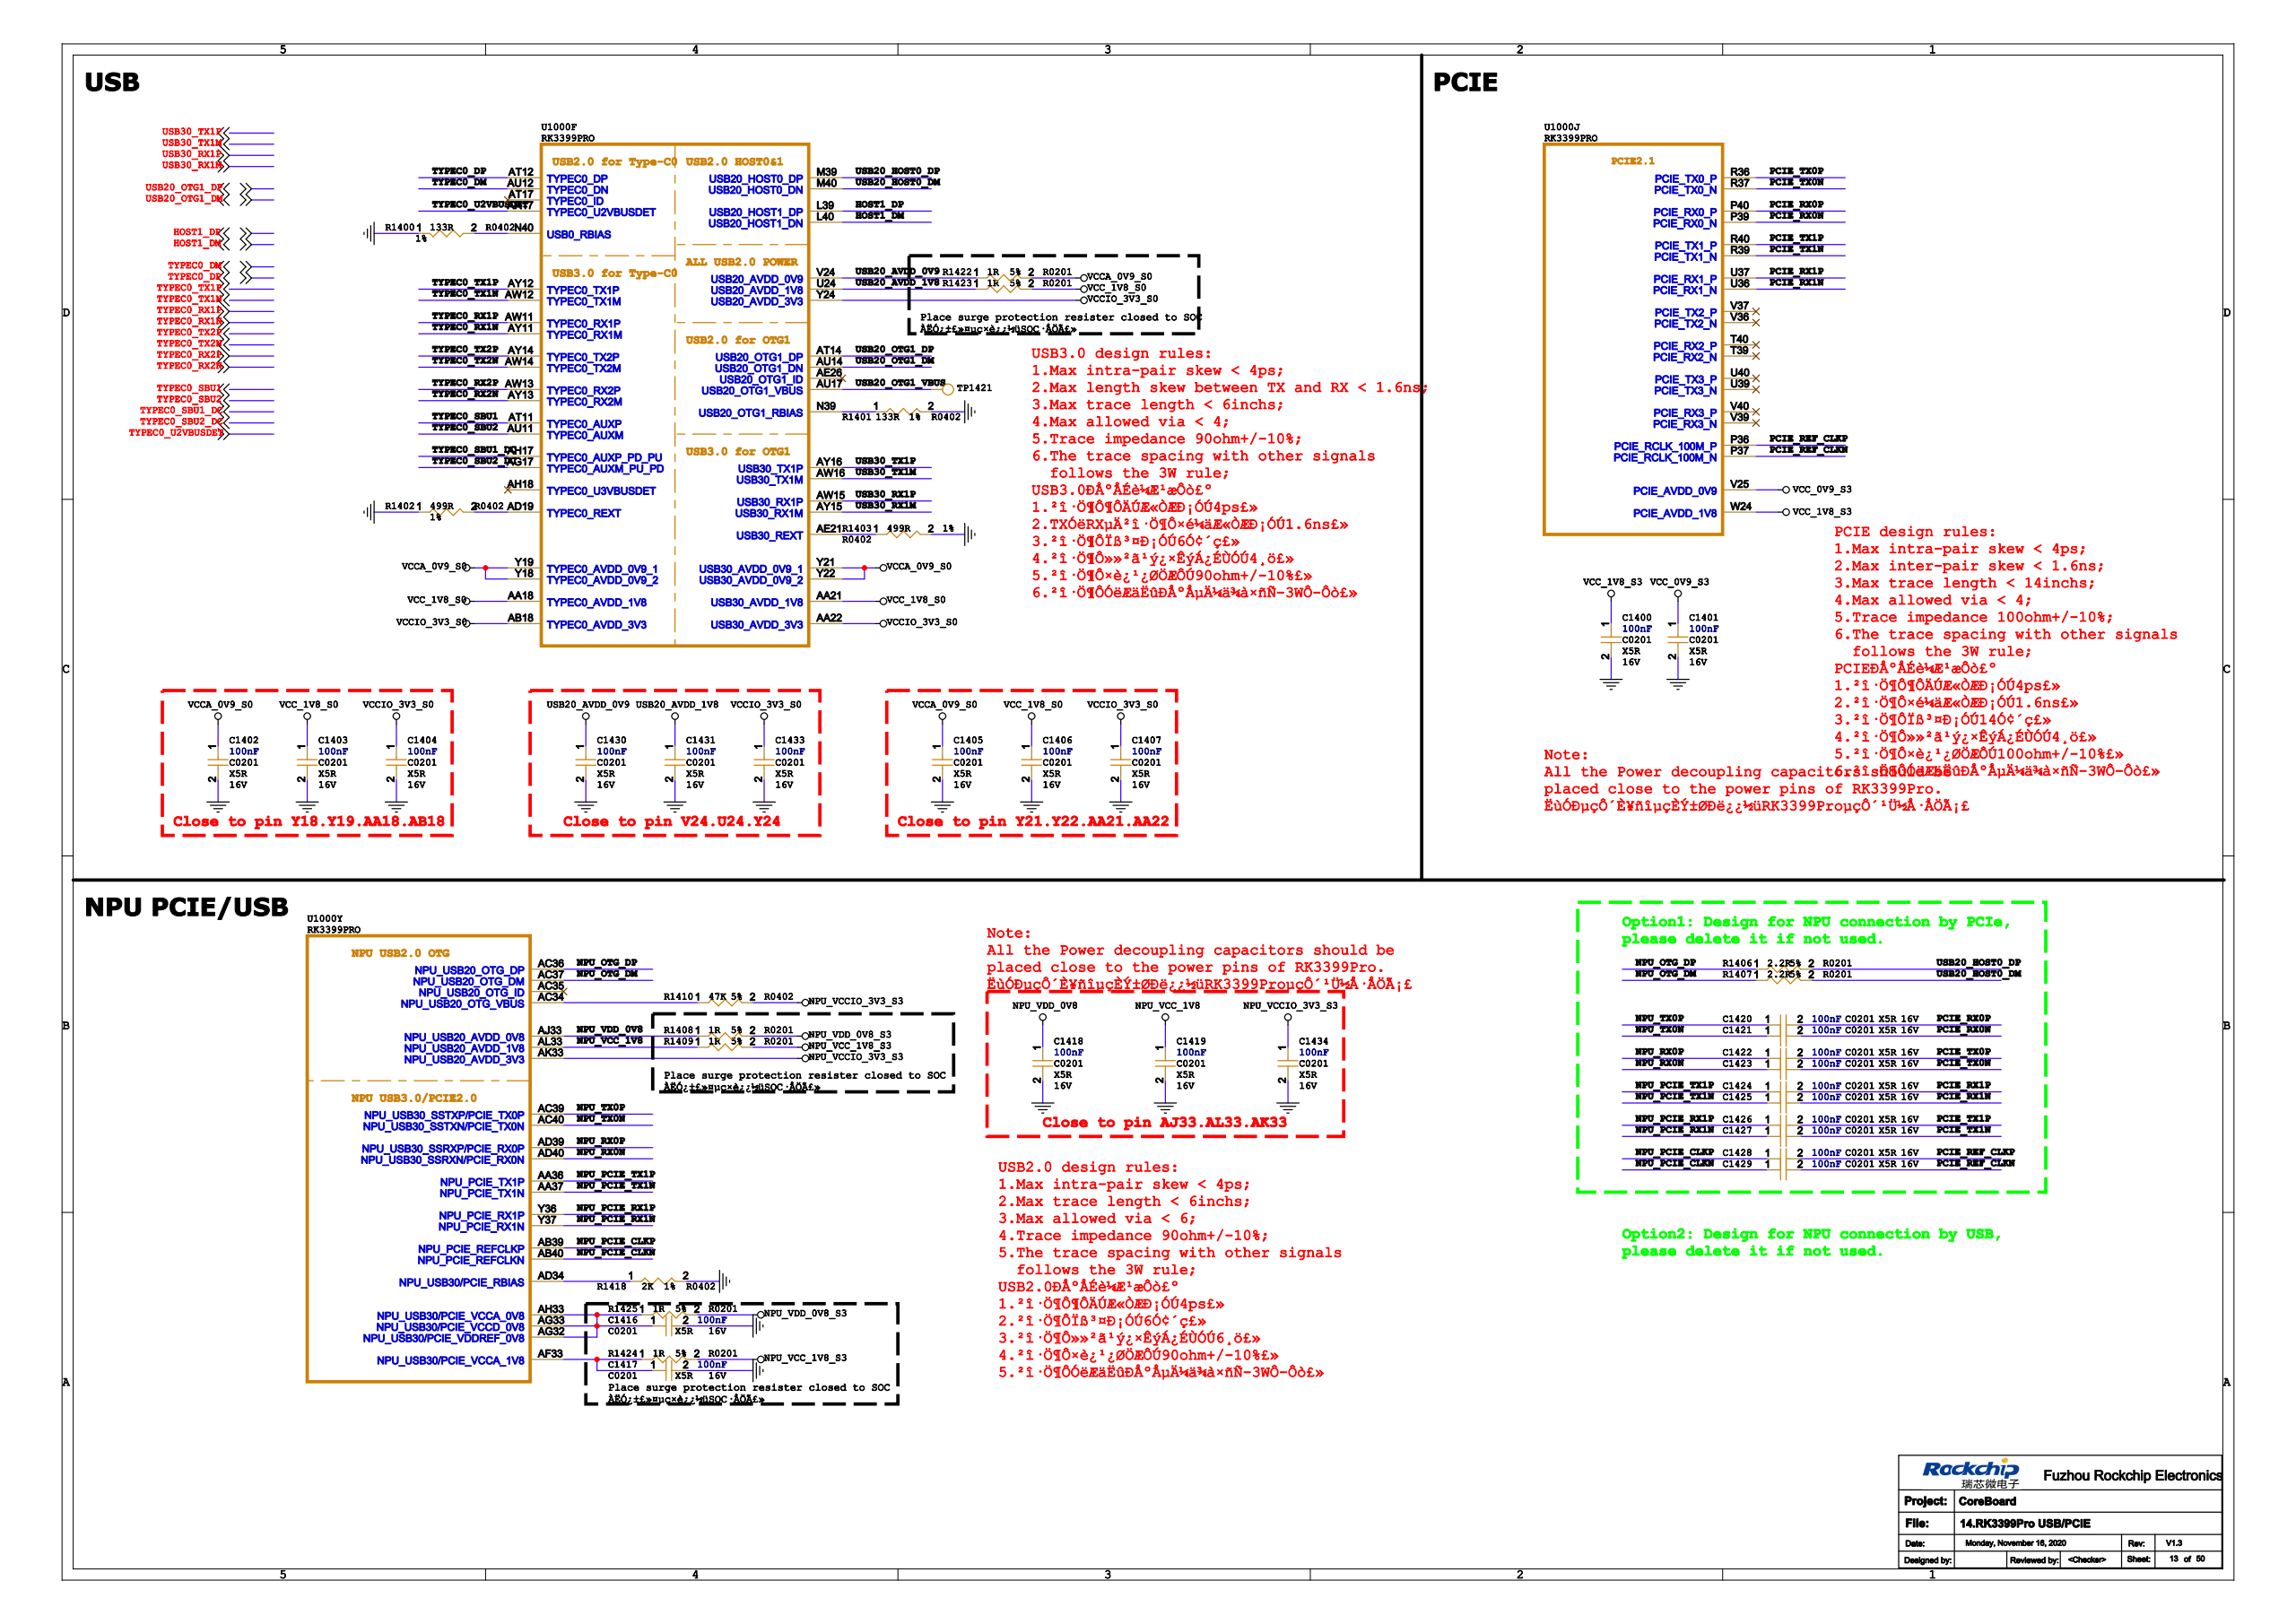Circuit board | Cadence Allegro | 749 parts | 717 nets | one sheet of the schematic
Parts on this sheet (reference | value | footprint):
C1400 | 100nF | C0201
C1401 | 100nF | C0201
C1402 | 100nF | C0201
C1403 | 100nF | C0201
C1404 | 100nF | C0201
C1405 | 100nF | C0201
C1406 | 100nF | C0201
C1407 | 100nF | C0201
C1416 | 100nF | C0201
C1417 | 100nF | C0201
C1418 | 100nF | C0201
C1419 | 100nF | C0201
C1420 | 100nF | C0201
C1421 | 100nF | C0201
C1422 | 100nF | C0201
C1423 | 100nF | C0201
C1424 | 100nF | C0201
C1425 | 100nF | C0201
C1426 | 100nF | C0201
C1427 | 100nF | C0201
C1428 | 100nF | C0201
C1429 | 100nF | C0201
C1430 | 100nF | C0201
C1431 | 100nF | C0201
C1433 | 100nF | C0201
C1434 | 100nF | C0201
R1400 | 133R | R0402
R1401 | 133R | R0402
R1402 | 499R | R0402
R1403 | 499R | R0402
R1418 | 2K | R0402
TP1421 | TP_0.5 | TP_0R50
U1000 | RK3399PRO | BGA1372_27R00X27R00X2R19
Nets of these parts (net: part-pin ...):
GND: C1400-2 C1401-2 C1402-2 C1403-2 C1404-2 C1405-2 C1406-2 C1407-2 C1416-2 C1417-2 C1418-2 C1419-2 C1430-2 C1431-2 C1433-2 C1434-2 R1400-1 R1401-2 R1402-1 R1403-2 R1418-2
TYPEC0_U2VBUSDET: U1000-AR17
TYPEC0_DP: U1000-AT12
USB20_OTG1_DM: U1000-AU14
TYPEC0_DM: U1000-AU12
USB20_OTG1_DP: U1000-AT14
USB30_RX1M: U1000-AY15
USB30_RX1P: U1000-AW15
TYPEC0_RX1P: U1000-AW11
USB30_TX1M: U1000-AW16
TYPEC0_RX1N: U1000-AY11
USB30_TX1P: U1000-AY16
VCC_1V8_S0: C1403-1 C1406-1 U1000-AA18 U1000-AA21
NPU_VCCIO_3V3_S3: C1434-1 U1000-AK33
TYPEC0_RX2P: U1000-AW13
TYPEC0_RX2N: U1000-AY13
HOST1_DM: U1000-L40
HOST1_DP: U1000-L39
VCCIO_3V3_S0: C1404-1 C1407-1 C1433-1 U1000-AA22 U1000-AB18 U1000-Y24
TYPEC0_SBU1_DC: U1000-AH17
TYPEC0_SBU2_DC: U1000-AG17
VCC_1V8_S3: C1400-1 U1000-W24
USB20_OTG1_VBUS: TP1421-1 U1000-AU17
VCC_0V9_S3: C1401-1 U1000-V25
N82549660: R1401-1 U1000-N39
USB20_AVDD_0V9: C1430-1 U1000-V24
USB20_AVDD_1V8: C1431-1 U1000-U24
USB20_HOST0_DM: U1000-M40
USB20_HOST0_DP: U1000-M39
VCCA_0V9_S0: C1402-1 C1405-1 U1000-Y18 U1000-Y19 U1000-Y21 U1000-Y22
N82550045: R1403-1 U1000-AE21
TYPEC0_SBU2: U1000-AU11
TYPEC0_SBU1: U1000-AT11
N82592823: R1402-2 U1000-AD19
TYPEC0_TX1N: U1000-AW12
TYPEC0_TX1P: U1000-AY12
TYPEC0_TX2N: U1000-AW14
TYPEC0_TX2P: U1000-AY14
N82592472: R1400-2 U1000-N40
PCIE_REF_CLKN: C1429-2 U1000-P37
PCIE_REF_CLKP: C1428-2 U1000-P36
PCIE_RX0N: C1421-2 U1000-P39
PCIE_RX0P: C1420-2 U1000-P40
PCIE_RX1N: C1425-2 U1000-U36
PCIE_RX1P: C1424-2 U1000-U37
PCIE_TX0N: C1423-2 U1000-R37
PCIE_TX0P: C1422-2 U1000-R36
PCIE_TX1N: C1427-2 U1000-R39
PCIE_TX1P: C1426-2 U1000-R40
N83929051: R1418-1 U1000-AD34
N83928853: C1416-1 U1000-AG32 U1000-AG33 U1000-AH33
N83928791: C1417-1 U1000-AF33
NPU_PCIE_CLKN: C1429-1 U1000-AB40
NPU_PCIE_CLKP: C1428-1 U1000-AB39
NPU_RX0N: C1423-1 U1000-AD40
NPU_RX0P: C1422-1 U1000-AD39
NPU_PCIE_RX1N: C1427-1 U1000-Y37
NPU_PCIE_RX1P: C1426-1 U1000-Y36
NPU_TX0N: C1421-1 U1000-AC40
NPU_TX0P: C1420-1 U1000-AC39
NPU_PCIE_TX1N: C1425-1 U1000-AA37
NPU_PCIE_TX1P: C1424-1 U1000-AA36
NPU_VDD_0V8: C1418-1 U1000-AJ33
NPU_VCC_1V8: C1419-1 U1000-AL33
NPU_OTG_DM: U1000-AC37
NPU_OTG_DP: U1000-AC36